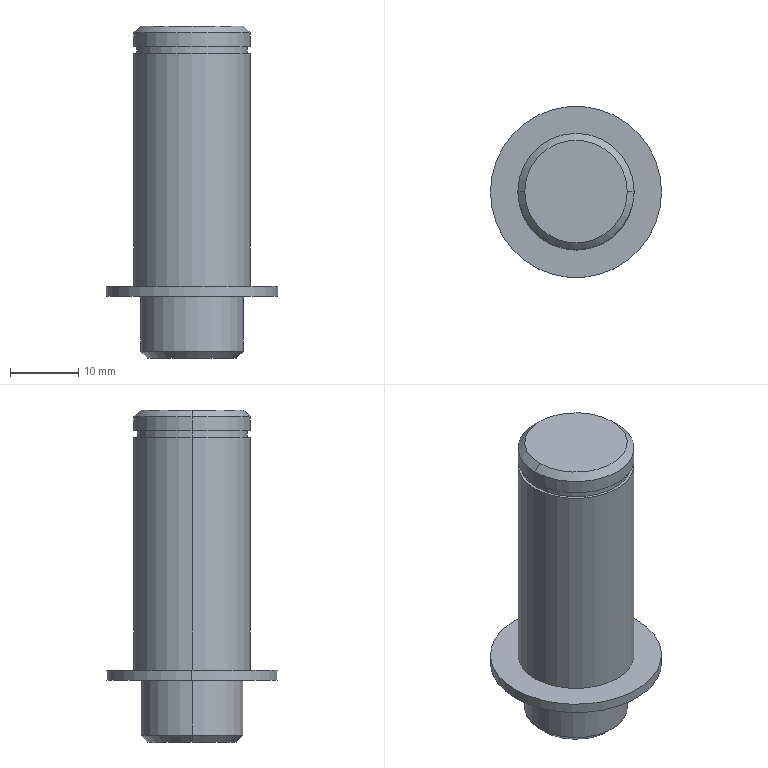Part | STEP file | CON-005 | 1 solid | 24 faces | box 25 x 25 x 48.5 mm | volume 10531 mm3 | cylinder 12 | cone 6 | plane 6 | commonest cylinder face diameters 17 x4 4.2 x2 15 x2 16.2 x2 25 x2
STEP:
#1=CARTESIAN_POINT('',(0.,0.,0.));
#2=DIRECTION('',(0.,0.,1.));
#3=DIRECTION('',(1.,0.,0.));
#4=AXIS2_PLACEMENT_3D('',#1,#2,#3);
#5=CARTESIAN_POINT('',(-6.5,0.,-44.5));
#6=VERTEX_POINT('',#5);
#7=CARTESIAN_POINT('',(6.5,0.,-44.5));
#8=VERTEX_POINT('',#7);
#9=CARTESIAN_POINT('',(0.,0.,-44.5));
#10=DIRECTION('',(0.,0.,-1.));
#11=DIRECTION('',(-1.,0.,0.));
#12=AXIS2_PLACEMENT_3D('',#9,#10,#11);
#13=CIRCLE('',#12,6.5);
#14=CARTESIAN_POINT('',(0.,0.,-44.5));
#15=DIRECTION('',(0.,0.,1.));
#16=DIRECTION('',(1.,0.,0.));
#17=AXIS2_PLACEMENT_3D('',#14,#15,#16);
#18=CONICAL_SURFACE('',#17,6.5,0.7854);
#19=CARTESIAN_POINT('',(3.142,0.));
#20=DIRECTION('',(-1.,0.));
#21=VECTOR('',#20,1.);
#22=LINE('',#19,#21);
#23=(GEOMETRIC_REPRESENTATION_CONTEXT(2)PARAMETRIC_REPRESENTATION_CONTEXT()REPRESENTATION_CONTEXT('',''));
#24=DEFINITIONAL_REPRESENTATION('',(#22),#23);
#25=PCURVE('',#18,#24);
#26=CARTESIAN_POINT('',(0.,0.,-44.5));
#27=DIRECTION('',(0.,0.,-1.));
#28=DIRECTION('',(-1.,0.,0.));
#29=AXIS2_PLACEMENT_3D('',#26,#27,#28);
#30=PLANE('',#29);
#31=CARTESIAN_POINT('',(0.,0.));
#32=DIRECTION('',(1.,0.));
#33=AXIS2_PLACEMENT_2D('',#31,#32);
#34=CIRCLE('',#33,6.5);
#35=(GEOMETRIC_REPRESENTATION_CONTEXT(2)PARAMETRIC_REPRESENTATION_CONTEXT()REPRESENTATION_CONTEXT('',''));
#36=DEFINITIONAL_REPRESENTATION('',(#34),#35);
#37=PCURVE('',#30,#36);
#38=SURFACE_CURVE('',#13,(#25,#37),.PCURVE_S1.);
#39=EDGE_CURVE('',#6,#8,#38,.T.);
#40=ORIENTED_EDGE('',*,*,#39,.F.);
#41=CARTESIAN_POINT('',(-7.5,0.,-43.5));
#42=VERTEX_POINT('',#41);
#43=CARTESIAN_POINT('',(-6.5,0.,-44.5));
#44=DIRECTION('',(-0.7071,0.,0.7071));
#45=VECTOR('',#44,1.);
#46=LINE('',#43,#45);
#47=CARTESIAN_POINT('',(3.142,0.));
#48=DIRECTION('',(0.,1.));
#49=VECTOR('',#48,1.);
#50=LINE('',#47,#49);
#51=(GEOMETRIC_REPRESENTATION_CONTEXT(2)PARAMETRIC_REPRESENTATION_CONTEXT()REPRESENTATION_CONTEXT('',''));
#52=DEFINITIONAL_REPRESENTATION('',(#50),#51);
#53=PCURVE('',#18,#52);
#54=CARTESIAN_POINT('',(0.,0.,-44.5));
#55=DIRECTION('',(0.,0.,1.));
#56=DIRECTION('',(1.,0.,0.));
#57=AXIS2_PLACEMENT_3D('',#54,#55,#56);
#58=CONICAL_SURFACE('',#57,6.5,0.7854);
#59=CARTESIAN_POINT('',(3.142,0.));
#60=DIRECTION('',(0.,1.));
#61=VECTOR('',#60,1.);
#62=LINE('',#59,#61);
#63=(GEOMETRIC_REPRESENTATION_CONTEXT(2)PARAMETRIC_REPRESENTATION_CONTEXT()REPRESENTATION_CONTEXT('',''));
#64=DEFINITIONAL_REPRESENTATION('',(#62),#63);
#65=PCURVE('',#58,#64);
#66=SURFACE_CURVE('',#46,(#53,#65),.PCURVE_S1.);
#67=EDGE_CURVE('',#6,#42,#66,.T.);
#68=ORIENTED_EDGE('',*,*,#67,.T.);
#69=CARTESIAN_POINT('',(7.5,0.,-43.5));
#70=VERTEX_POINT('',#69);
#71=CARTESIAN_POINT('',(0.,0.,-43.5));
#72=DIRECTION('',(0.,0.,1.));
#73=DIRECTION('',(-1.,0.,0.));
#74=AXIS2_PLACEMENT_3D('',#71,#72,#73);
#75=CIRCLE('',#74,7.5);
#76=CARTESIAN_POINT('',(-3.142,1.));
#77=DIRECTION('',(1.,0.));
#78=VECTOR('',#77,1.);
#79=LINE('',#76,#78);
#80=(GEOMETRIC_REPRESENTATION_CONTEXT(2)PARAMETRIC_REPRESENTATION_CONTEXT()REPRESENTATION_CONTEXT('',''));
#81=DEFINITIONAL_REPRESENTATION('',(#79),#80);
#82=PCURVE('',#18,#81);
#83=CARTESIAN_POINT('',(0.,0.,-44.5));
#84=DIRECTION('',(0.,0.,1.));
#85=DIRECTION('',(1.,0.,0.));
#86=AXIS2_PLACEMENT_3D('',#83,#84,#85);
#87=CYLINDRICAL_SURFACE('',#86,7.5);
#88=CARTESIAN_POINT('',(-3.142,1.));
#89=DIRECTION('',(1.,0.));
#90=VECTOR('',#89,1.);
#91=LINE('',#88,#90);
#92=(GEOMETRIC_REPRESENTATION_CONTEXT(2)PARAMETRIC_REPRESENTATION_CONTEXT()REPRESENTATION_CONTEXT('',''));
#93=DEFINITIONAL_REPRESENTATION('',(#91),#92);
#94=PCURVE('',#87,#93);
#95=SURFACE_CURVE('',#75,(#82,#94),.PCURVE_S1.);
#96=EDGE_CURVE('',#70,#42,#95,.T.);
#97=ORIENTED_EDGE('',*,*,#96,.F.);
#98=CARTESIAN_POINT('',(6.5,0.,-44.5));
#99=DIRECTION('',(0.7071,0.,0.7071));
#100=VECTOR('',#99,1.);
#101=LINE('',#98,#100);
#102=CARTESIAN_POINT('',(0.,0.));
#103=DIRECTION('',(0.,1.));
#104=VECTOR('',#103,1.);
#105=LINE('',#102,#104);
#106=(GEOMETRIC_REPRESENTATION_CONTEXT(2)PARAMETRIC_REPRESENTATION_CONTEXT()REPRESENTATION_CONTEXT('',''));
#107=DEFINITIONAL_REPRESENTATION('',(#105),#106);
#108=PCURVE('',#18,#107);
#109=CARTESIAN_POINT('',(6.283,0.));
#110=DIRECTION('',(0.,1.));
#111=VECTOR('',#110,1.);
#112=LINE('',#109,#111);
#113=(GEOMETRIC_REPRESENTATION_CONTEXT(2)PARAMETRIC_REPRESENTATION_CONTEXT()REPRESENTATION_CONTEXT('',''));
#114=DEFINITIONAL_REPRESENTATION('',(#112),#113);
#115=PCURVE('',#58,#114);
#116=SURFACE_CURVE('',#101,(#108,#115),.PCURVE_S1.);
#117=EDGE_CURVE('',#8,#70,#116,.T.);
#118=ORIENTED_EDGE('',*,*,#117,.F.);
#119=EDGE_LOOP('',(#40,#68,#97,#118));
#120=FACE_BOUND('',#119,.T.);
#121=ADVANCED_FACE('',(#120),#18,.T.);
#122=CARTESIAN_POINT('',(7.5,0.,4.));
#123=VERTEX_POINT('',#122);
#124=CARTESIAN_POINT('',(-7.5,0.,4.));
#125=VERTEX_POINT('',#124);
#126=CARTESIAN_POINT('',(0.,0.,4.));
#127=DIRECTION('',(0.,0.,1.));
#128=DIRECTION('',(1.,0.,0.));
#129=AXIS2_PLACEMENT_3D('',#126,#127,#128);
#130=CIRCLE('',#129,7.5);
#131=CARTESIAN_POINT('',(0.,0.,4.));
#132=DIRECTION('',(0.,0.,-1.));
#133=DIRECTION('',(-1.,0.,0.));
#134=AXIS2_PLACEMENT_3D('',#131,#132,#133);
#135=CONICAL_SURFACE('',#134,7.5,0.7854);
#136=CARTESIAN_POINT('',(3.142,0.));
#137=DIRECTION('',(-1.,0.));
#138=VECTOR('',#137,1.);
#139=LINE('',#136,#138);
#140=(GEOMETRIC_REPRESENTATION_CONTEXT(2)PARAMETRIC_REPRESENTATION_CONTEXT()REPRESENTATION_CONTEXT('',''));
#141=DEFINITIONAL_REPRESENTATION('',(#139),#140);
#142=PCURVE('',#135,#141);
#143=CARTESIAN_POINT('',(0.,0.,4.));
#144=DIRECTION('',(0.,0.,1.));
#145=DIRECTION('',(1.,0.,0.));
#146=AXIS2_PLACEMENT_3D('',#143,#144,#145);
#147=PLANE('',#146);
#148=CARTESIAN_POINT('',(0.,0.));
#149=DIRECTION('',(1.,0.));
#150=AXIS2_PLACEMENT_2D('',#148,#149);
#151=CIRCLE('',#150,7.5);
#152=(GEOMETRIC_REPRESENTATION_CONTEXT(2)PARAMETRIC_REPRESENTATION_CONTEXT()REPRESENTATION_CONTEXT('',''));
#153=DEFINITIONAL_REPRESENTATION('',(#151),#152);
#154=PCURVE('',#147,#153);
#155=SURFACE_CURVE('',#130,(#142,#154),.PCURVE_S1.);
#156=EDGE_CURVE('',#123,#125,#155,.T.);
#157=ORIENTED_EDGE('',*,*,#156,.F.);
#158=CARTESIAN_POINT('',(8.5,0.,3.));
#159=VERTEX_POINT('',#158);
#160=CARTESIAN_POINT('',(7.5,0.,4.));
#161=DIRECTION('',(0.7071,0.,-0.7071));
#162=VECTOR('',#161,1.);
#163=LINE('',#160,#162);
#164=CARTESIAN_POINT('',(3.142,0.));
#165=DIRECTION('',(0.,1.));
#166=VECTOR('',#165,1.);
#167=LINE('',#164,#166);
#168=(GEOMETRIC_REPRESENTATION_CONTEXT(2)PARAMETRIC_REPRESENTATION_CONTEXT()REPRESENTATION_CONTEXT('',''));
#169=DEFINITIONAL_REPRESENTATION('',(#167),#168);
#170=PCURVE('',#135,#169);
#171=CARTESIAN_POINT('',(0.,0.,4.));
#172=DIRECTION('',(0.,0.,-1.));
#173=DIRECTION('',(-1.,0.,0.));
#174=AXIS2_PLACEMENT_3D('',#171,#172,#173);
#175=CONICAL_SURFACE('',#174,7.5,0.7854);
#176=CARTESIAN_POINT('',(3.142,0.));
#177=DIRECTION('',(0.,1.));
#178=VECTOR('',#177,1.);
#179=LINE('',#176,#178);
#180=(GEOMETRIC_REPRESENTATION_CONTEXT(2)PARAMETRIC_REPRESENTATION_CONTEXT()REPRESENTATION_CONTEXT('',''));
#181=DEFINITIONAL_REPRESENTATION('',(#179),#180);
#182=PCURVE('',#175,#181);
#183=SURFACE_CURVE('',#163,(#170,#182),.PCURVE_S1.);
#184=EDGE_CURVE('',#123,#159,#183,.T.);
#185=ORIENTED_EDGE('',*,*,#184,.T.);
#186=CARTESIAN_POINT('',(-8.5,0.,3.));
#187=VERTEX_POINT('',#186);
#188=CARTESIAN_POINT('',(0.,0.,3.));
#189=DIRECTION('',(0.,0.,-1.));
#190=DIRECTION('',(1.,0.,0.));
#191=AXIS2_PLACEMENT_3D('',#188,#189,#190);
#192=CIRCLE('',#191,8.5);
#193=CARTESIAN_POINT('',(-3.142,1.));
#194=DIRECTION('',(1.,0.));
#195=VECTOR('',#194,1.);
#196=LINE('',#193,#195);
#197=(GEOMETRIC_REPRESENTATION_CONTEXT(2)PARAMETRIC_REPRESENTATION_CONTEXT()REPRESENTATION_CONTEXT('',''));
#198=DEFINITIONAL_REPRESENTATION('',(#196),#197);
#199=PCURVE('',#135,#198);
#200=CARTESIAN_POINT('',(0.,0.,4.));
#201=DIRECTION('',(0.,0.,-1.));
#202=DIRECTION('',(-1.,0.,0.));
#203=AXIS2_PLACEMENT_3D('',#200,#201,#202);
#204=CYLINDRICAL_SURFACE('',#203,8.5);
#205=CARTESIAN_POINT('',(-3.142,1.));
#206=DIRECTION('',(1.,0.));
#207=VECTOR('',#206,1.);
#208=LINE('',#205,#207);
#209=(GEOMETRIC_REPRESENTATION_CONTEXT(2)PARAMETRIC_REPRESENTATION_CONTEXT()REPRESENTATION_CONTEXT('',''));
#210=DEFINITIONAL_REPRESENTATION('',(#208),#209);
#211=PCURVE('',#204,#210);
#212=SURFACE_CURVE('',#192,(#199,#211),.PCURVE_S1.);
#213=EDGE_CURVE('',#187,#159,#212,.T.);
#214=ORIENTED_EDGE('',*,*,#213,.F.);
#215=CARTESIAN_POINT('',(-7.5,0.,4.));
#216=DIRECTION('',(-0.7071,0.,-0.7071));
#217=VECTOR('',#216,1.);
#218=LINE('',#215,#217);
#219=CARTESIAN_POINT('',(0.,0.));
#220=DIRECTION('',(0.,1.));
#221=VECTOR('',#220,1.);
#222=LINE('',#219,#221);
#223=(GEOMETRIC_REPRESENTATION_CONTEXT(2)PARAMETRIC_REPRESENTATION_CONTEXT()REPRESENTATION_CONTEXT('',''));
#224=DEFINITIONAL_REPRESENTATION('',(#222),#223);
#225=PCURVE('',#135,#224);
#226=CARTESIAN_POINT('',(6.283,0.));
#227=DIRECTION('',(0.,1.));
#228=VECTOR('',#227,1.);
#229=LINE('',#226,#228);
#230=(GEOMETRIC_REPRESENTATION_CONTEXT(2)PARAMETRIC_REPRESENTATION_CONTEXT()REPRESENTATION_CONTEXT('',''));
#231=DEFINITIONAL_REPRESENTATION('',(#229),#230);
#232=PCURVE('',#175,#231);
#233=SURFACE_CURVE('',#218,(#225,#232),.PCURVE_S1.);
#234=EDGE_CURVE('',#125,#187,#233,.T.);
#235=ORIENTED_EDGE('',*,*,#234,.F.);
#236=EDGE_LOOP('',(#157,#185,#214,#235));
#237=FACE_BOUND('',#236,.T.);
#238=ADVANCED_FACE('',(#237),#135,.T.);
#239=CARTESIAN_POINT('',(-2.1,0.,-19.5));
#240=VERTEX_POINT('',#239);
#241=CARTESIAN_POINT('',(-2.1,0.,-44.5));
#242=VERTEX_POINT('',#241);
#243=CARTESIAN_POINT('',(-2.1,0.,-44.5));
#244=DIRECTION('',(0.,0.,-1.));
#245=VECTOR('',#244,1.);
#246=LINE('',#243,#245);
#247=CARTESIAN_POINT('',(0.,0.,-44.5));
#248=DIRECTION('',(0.,0.,-1.));
#249=DIRECTION('',(-1.,0.,0.));
#250=AXIS2_PLACEMENT_3D('',#247,#248,#249);
#251=CYLINDRICAL_SURFACE('',#250,2.1);
#252=CARTESIAN_POINT('',(6.283,0.));
#253=DIRECTION('',(0.,1.));
#254=VECTOR('',#253,1.);
#255=LINE('',#252,#254);
#256=(GEOMETRIC_REPRESENTATION_CONTEXT(2)PARAMETRIC_REPRESENTATION_CONTEXT()REPRESENTATION_CONTEXT('',''));
#257=DEFINITIONAL_REPRESENTATION('',(#255),#256);
#258=PCURVE('',#251,#257);
#259=CARTESIAN_POINT('',(0.,0.,-44.5));
#260=DIRECTION('',(0.,0.,-1.));
#261=DIRECTION('',(-1.,0.,0.));
#262=AXIS2_PLACEMENT_3D('',#259,#260,#261);
#263=CYLINDRICAL_SURFACE('',#262,2.1);
#264=CARTESIAN_POINT('',(0.,0.));
#265=DIRECTION('',(0.,1.));
#266=VECTOR('',#265,1.);
#267=LINE('',#264,#266);
#268=(GEOMETRIC_REPRESENTATION_CONTEXT(2)PARAMETRIC_REPRESENTATION_CONTEXT()REPRESENTATION_CONTEXT('',''));
#269=DEFINITIONAL_REPRESENTATION('',(#267),#268);
#270=PCURVE('',#263,#269);
#271=SURFACE_CURVE('',#246,(#258,#270),.PCURVE_S1.);
#272=EDGE_CURVE('',#240,#242,#271,.T.);
#273=ORIENTED_EDGE('',*,*,#272,.T.);
#274=CARTESIAN_POINT('',(2.1,0.,-44.5));
#275=VERTEX_POINT('',#274);
#276=CARTESIAN_POINT('',(0.,0.,-44.5));
#277=DIRECTION('',(0.,0.,-1.));
#278=DIRECTION('',(-1.,0.,0.));
#279=AXIS2_PLACEMENT_3D('',#276,#277,#278);
#280=CIRCLE('',#279,2.1);
#281=CARTESIAN_POINT('',(0.,0.));
#282=DIRECTION('',(1.,0.));
#283=VECTOR('',#282,1.);
#284=LINE('',#281,#283);
#285=(GEOMETRIC_REPRESENTATION_CONTEXT(2)PARAMETRIC_REPRESENTATION_CONTEXT()REPRESENTATION_CONTEXT('',''));
#286=DEFINITIONAL_REPRESENTATION('',(#284),#285);
#287=PCURVE('',#251,#286);
#288=CARTESIAN_POINT('',(0.,0.));
#289=DIRECTION('',(1.,0.));
#290=AXIS2_PLACEMENT_2D('',#288,#289);
#291=CIRCLE('',#290,2.1);
#292=(GEOMETRIC_REPRESENTATION_CONTEXT(2)PARAMETRIC_REPRESENTATION_CONTEXT()REPRESENTATION_CONTEXT('',''));
#293=DEFINITIONAL_REPRESENTATION('',(#291),#292);
#294=PCURVE('',#30,#293);
#295=SURFACE_CURVE('',#280,(#287,#294),.PCURVE_S1.);
#296=EDGE_CURVE('',#275,#242,#295,.T.);
#297=ORIENTED_EDGE('',*,*,#296,.F.);
#298=CARTESIAN_POINT('',(2.1,0.,-19.5));
#299=VERTEX_POINT('',#298);
#300=CARTESIAN_POINT('',(2.1,0.,-44.5));
#301=DIRECTION('',(0.,0.,-1.));
#302=VECTOR('',#301,1.);
#303=LINE('',#300,#302);
#304=CARTESIAN_POINT('',(3.142,0.));
#305=DIRECTION('',(0.,1.));
#306=VECTOR('',#305,1.);
#307=LINE('',#304,#306);
#308=(GEOMETRIC_REPRESENTATION_CONTEXT(2)PARAMETRIC_REPRESENTATION_CONTEXT()REPRESENTATION_CONTEXT('',''));
#309=DEFINITIONAL_REPRESENTATION('',(#307),#308);
#310=PCURVE('',#251,#309);
#311=CARTESIAN_POINT('',(3.142,0.));
#312=DIRECTION('',(0.,1.));
#313=VECTOR('',#312,1.);
#314=LINE('',#311,#313);
#315=(GEOMETRIC_REPRESENTATION_CONTEXT(2)PARAMETRIC_REPRESENTATION_CONTEXT()REPRESENTATION_CONTEXT('',''));
#316=DEFINITIONAL_REPRESENTATION('',(#314),#315);
#317=PCURVE('',#263,#316);
#318=SURFACE_CURVE('',#303,(#310,#317),.PCURVE_S1.);
#319=EDGE_CURVE('',#299,#275,#318,.T.);
#320=ORIENTED_EDGE('',*,*,#319,.F.);
#321=CARTESIAN_POINT('',(0.,0.,-19.5));
#322=DIRECTION('',(0.,0.,-1.));
#323=DIRECTION('',(-1.,0.,0.));
#324=AXIS2_PLACEMENT_3D('',#321,#322,#323);
#325=CIRCLE('',#324,2.1);
#326=CARTESIAN_POINT('',(0.,-25.));
#327=DIRECTION('',(1.,0.));
#328=VECTOR('',#327,1.);
#329=LINE('',#326,#328);
#330=(GEOMETRIC_REPRESENTATION_CONTEXT(2)PARAMETRIC_REPRESENTATION_CONTEXT()REPRESENTATION_CONTEXT('',''));
#331=DEFINITIONAL_REPRESENTATION('',(#329),#330);
#332=PCURVE('',#251,#331);
#333=CARTESIAN_POINT('',(0.,0.,-19.5));
#334=DIRECTION('',(0.,0.,-1.));
#335=DIRECTION('',(-1.,0.,0.));
#336=AXIS2_PLACEMENT_3D('',#333,#334,#335);
#337=CONICAL_SURFACE('',#336,2.1,1.03);
#338=CARTESIAN_POINT('',(0.,0.));
#339=DIRECTION('',(1.,0.));
#340=VECTOR('',#339,1.);
#341=LINE('',#338,#340);
#342=(GEOMETRIC_REPRESENTATION_CONTEXT(2)PARAMETRIC_REPRESENTATION_CONTEXT()REPRESENTATION_CONTEXT('',''));
#343=DEFINITIONAL_REPRESENTATION('',(#341),#342);
#344=PCURVE('',#337,#343);
#345=SURFACE_CURVE('',#325,(#332,#344),.PCURVE_S1.);
#346=EDGE_CURVE('',#299,#240,#345,.T.);
#347=ORIENTED_EDGE('',*,*,#346,.T.);
#348=EDGE_LOOP('',(#273,#297,#320,#347));
#349=FACE_BOUND('',#348,.F.);
#350=ADVANCED_FACE('',(#349),#251,.F.);
#351=ORIENTED_EDGE('',*,*,#346,.F.);
#352=CARTESIAN_POINT('',(0.,0.,-18.238));
#353=VERTEX_POINT('',#352);
#354=CARTESIAN_POINT('',(2.1,0.,-19.5));
#355=DIRECTION('',(0.8572,0.,-0.515));
#356=VECTOR('',#355,1.);
#357=LINE('',#354,#356);
#358=CARTESIAN_POINT('',(3.142,0.));
#359=DIRECTION('',(0.,1.));
#360=VECTOR('',#359,1.);
#361=LINE('',#358,#360);
#362=(GEOMETRIC_REPRESENTATION_CONTEXT(2)PARAMETRIC_REPRESENTATION_CONTEXT()REPRESENTATION_CONTEXT('',''));
#363=DEFINITIONAL_REPRESENTATION('',(#361),#362);
#364=PCURVE('',#337,#363);
#365=CARTESIAN_POINT('',(0.,0.,-19.5));
#366=DIRECTION('',(0.,0.,-1.));
#367=DIRECTION('',(-1.,0.,0.));
#368=AXIS2_PLACEMENT_3D('',#365,#366,#367);
#369=CONICAL_SURFACE('',#368,2.1,1.03);
#370=CARTESIAN_POINT('',(3.142,0.));
#371=DIRECTION('',(0.,1.));
#372=VECTOR('',#371,1.);
#373=LINE('',#370,#372);
#374=(GEOMETRIC_REPRESENTATION_CONTEXT(2)PARAMETRIC_REPRESENTATION_CONTEXT()REPRESENTATION_CONTEXT('',''));
#375=DEFINITIONAL_REPRESENTATION('',(#373),#374);
#376=PCURVE('',#369,#375);
#377=SURFACE_CURVE('',#357,(#364,#376),.PCURVE_S1.);
#378=EDGE_CURVE('',#353,#299,#377,.T.);
#379=ORIENTED_EDGE('',*,*,#378,.F.);
#380=CARTESIAN_POINT('',(-2.1,0.,-19.5));
#381=DIRECTION('',(-0.8572,0.,-0.515));
#382=VECTOR('',#381,1.);
#383=LINE('',#380,#382);
#384=CARTESIAN_POINT('',(6.283,0.));
#385=DIRECTION('',(0.,1.));
#386=VECTOR('',#385,1.);
#387=LINE('',#384,#386);
#388=(GEOMETRIC_REPRESENTATION_CONTEXT(2)PARAMETRIC_REPRESENTATION_CONTEXT()REPRESENTATION_CONTEXT('',''));
#389=DEFINITIONAL_REPRESENTATION('',(#387),#388);
#390=PCURVE('',#337,#389);
#391=CARTESIAN_POINT('',(0.,0.));
#392=DIRECTION('',(0.,1.));
#393=VECTOR('',#392,1.);
#394=LINE('',#391,#393);
#395=(GEOMETRIC_REPRESENTATION_CONTEXT(2)PARAMETRIC_REPRESENTATION_CONTEXT()REPRESENTATION_CONTEXT('',''));
#396=DEFINITIONAL_REPRESENTATION('',(#394),#395);
#397=PCURVE('',#369,#396);
#398=SURFACE_CURVE('',#383,(#390,#397),.PCURVE_S1.);
#399=EDGE_CURVE('',#353,#240,#398,.T.);
#400=ORIENTED_EDGE('',*,*,#399,.T.);
#401=EDGE_LOOP('',(#351,#379,#400));
#402=FACE_BOUND('',#401,.F.);
#403=ADVANCED_FACE('',(#402),#337,.F.);
#404=ORIENTED_EDGE('',*,*,#213,.T.);
#405=CARTESIAN_POINT('',(8.5,0.,1.));
#406=VERTEX_POINT('',#405);
#407=CARTESIAN_POINT('',(8.5,0.,4.));
#408=DIRECTION('',(0.,0.,-1.));
#409=VECTOR('',#408,1.);
#410=LINE('',#407,#409);
#411=CARTESIAN_POINT('',(3.142,0.));
#412=DIRECTION('',(0.,1.));
#413=VECTOR('',#412,1.);
#414=LINE('',#411,#413);
#415=(GEOMETRIC_REPRESENTATION_CONTEXT(2)PARAMETRIC_REPRESENTATION_CONTEXT()REPRESENTATION_CONTEXT('',''));
#416=DEFINITIONAL_REPRESENTATION('',(#414),#415);
#417=PCURVE('',#204,#416);
#418=CARTESIAN_POINT('',(0.,0.,4.));
#419=DIRECTION('',(0.,0.,-1.));
#420=DIRECTION('',(-1.,0.,0.));
#421=AXIS2_PLACEMENT_3D('',#418,#419,#420);
#422=CYLINDRICAL_SURFACE('',#421,8.5);
#423=CARTESIAN_POINT('',(3.142,0.));
#424=DIRECTION('',(0.,1.));
#425=VECTOR('',#424,1.);
#426=LINE('',#423,#425);
#427=(GEOMETRIC_REPRESENTATION_CONTEXT(2)PARAMETRIC_REPRESENTATION_CONTEXT()REPRESENTATION_CONTEXT('',''));
#428=DEFINITIONAL_REPRESENTATION('',(#426),#427);
#429=PCURVE('',#422,#428);
#430=SURFACE_CURVE('',#410,(#417,#429),.PCURVE_S1.);
#431=EDGE_CURVE('',#159,#406,#430,.T.);
#432=ORIENTED_EDGE('',*,*,#431,.T.);
#433=CARTESIAN_POINT('',(-8.5,0.,1.));
#434=VERTEX_POINT('',#433);
#435=CARTESIAN_POINT('',(0.,0.,1.));
#436=DIRECTION('',(0.,0.,1.));
#437=DIRECTION('',(1.,0.,0.));
#438=AXIS2_PLACEMENT_3D('',#435,#436,#437);
#439=CIRCLE('',#438,8.5);
#440=CARTESIAN_POINT('',(3.142,3.));
#441=DIRECTION('',(-1.,0.));
#442=VECTOR('',#441,1.);
#443=LINE('',#440,#442);
#444=(GEOMETRIC_REPRESENTATION_CONTEXT(2)PARAMETRIC_REPRESENTATION_CONTEXT()REPRESENTATION_CONTEXT('',''));
#445=DEFINITIONAL_REPRESENTATION('',(#443),#444);
#446=PCURVE('',#204,#445);
#447=CARTESIAN_POINT('',(0.,0.,1.));
#448=DIRECTION('',(0.,0.,1.));
#449=DIRECTION('',(1.,0.,0.));
#450=AXIS2_PLACEMENT_3D('',#447,#448,#449);
#451=PLANE('',#450);
#452=CARTESIAN_POINT('',(0.,0.));
#453=DIRECTION('',(1.,0.));
#454=AXIS2_PLACEMENT_2D('',#452,#453);
#455=CIRCLE('',#454,8.5);
#456=(GEOMETRIC_REPRESENTATION_CONTEXT(2)PARAMETRIC_REPRESENTATION_CONTEXT()REPRESENTATION_CONTEXT('',''));
#457=DEFINITIONAL_REPRESENTATION('',(#455),#456);
#458=PCURVE('',#451,#457);
#459=SURFACE_CURVE('',#439,(#446,#458),.PCURVE_S1.);
#460=EDGE_CURVE('',#406,#434,#459,.T.);
#461=ORIENTED_EDGE('',*,*,#460,.T.);
#462=CARTESIAN_POINT('',(-8.5,0.,4.));
#463=DIRECTION('',(0.,0.,-1.));
#464=VECTOR('',#463,1.);
#465=LINE('',#462,#464);
#466=CARTESIAN_POINT('',(0.,0.));
#467=DIRECTION('',(0.,1.));
#468=VECTOR('',#467,1.);
#469=LINE('',#466,#468);
#470=(GEOMETRIC_REPRESENTATION_CONTEXT(2)PARAMETRIC_REPRESENTATION_CONTEXT()REPRESENTATION_CONTEXT('',''));
#471=DEFINITIONAL_REPRESENTATION('',(#469),#470);
#472=PCURVE('',#204,#471);
#473=CARTESIAN_POINT('',(6.283,0.));
#474=DIRECTION('',(0.,1.));
#475=VECTOR('',#474,1.);
#476=LINE('',#473,#475);
#477=(GEOMETRIC_REPRESENTATION_CONTEXT(2)PARAMETRIC_REPRESENTATION_CONTEXT()REPRESENTATION_CONTEXT('',''));
#478=DEFINITIONAL_REPRESENTATION('',(#476),#477);
#479=PCURVE('',#422,#478);
#480=SURFACE_CURVE('',#465,(#472,#479),.PCURVE_S1.);
#481=EDGE_CURVE('',#187,#434,#480,.T.);
#482=ORIENTED_EDGE('',*,*,#481,.F.);
#483=EDGE_LOOP('',(#404,#432,#461,#482));
#484=FACE_BOUND('',#483,.T.);
#485=ADVANCED_FACE('',(#484),#204,.T.);
#486=CARTESIAN_POINT('',(8.1,0.,1.));
#487=VERTEX_POINT('',#486);
#488=CARTESIAN_POINT('',(-8.1,0.,1.));
#489=VERTEX_POINT('',#488);
#490=CARTESIAN_POINT('',(0.,0.,1.));
#491=DIRECTION('',(0.,0.,1.));
#492=DIRECTION('',(1.,0.,0.));
#493=AXIS2_PLACEMENT_3D('',#490,#491,#492);
#494=CIRCLE('',#493,8.1);
#495=CARTESIAN_POINT('',(0.,0.,1.));
#496=DIRECTION('',(0.,0.,-1.));
#497=DIRECTION('',(-1.,0.,0.));
#498=AXIS2_PLACEMENT_3D('',#495,#496,#497);
#499=CYLINDRICAL_SURFACE('',#498,8.1);
#500=CARTESIAN_POINT('',(3.142,0.));
#501=DIRECTION('',(-1.,0.));
#502=VECTOR('',#501,1.);
#503=LINE('',#500,#502);
#504=(GEOMETRIC_REPRESENTATION_CONTEXT(2)PARAMETRIC_REPRESENTATION_CONTEXT()REPRESENTATION_CONTEXT('',''));
#505=DEFINITIONAL_REPRESENTATION('',(#503),#504);
#506=PCURVE('',#499,#505);
#507=CARTESIAN_POINT('',(0.,0.));
#508=DIRECTION('',(1.,0.));
#509=AXIS2_PLACEMENT_2D('',#507,#508);
#510=CIRCLE('',#509,8.1);
#511=(GEOMETRIC_REPRESENTATION_CONTEXT(2)PARAMETRIC_REPRESENTATION_CONTEXT()REPRESENTATION_CONTEXT('',''));
#512=DEFINITIONAL_REPRESENTATION('',(#510),#511);
#513=PCURVE('',#451,#512);
#514=SURFACE_CURVE('',#494,(#506,#513),.PCURVE_S1.);
#515=EDGE_CURVE('',#487,#489,#514,.T.);
#516=ORIENTED_EDGE('',*,*,#515,.F.);
#517=CARTESIAN_POINT('',(8.1,0.,0.));
#518=VERTEX_POINT('',#517);
#519=CARTESIAN_POINT('',(8.1,0.,1.));
#520=DIRECTION('',(0.,0.,-1.));
#521=VECTOR('',#520,1.);
#522=LINE('',#519,#521);
#523=CARTESIAN_POINT('',(3.142,0.));
#524=DIRECTION('',(0.,1.));
#525=VECTOR('',#524,1.);
#526=LINE('',#523,#525);
#527=(GEOMETRIC_REPRESENTATION_CONTEXT(2)PARAMETRIC_REPRESENTATION_CONTEXT()REPRESENTATION_CONTEXT('',''));
#528=DEFINITIONAL_REPRESENTATION('',(#526),#527);
#529=PCURVE('',#499,#528);
#530=CARTESIAN_POINT('',(0.,0.,1.));
#531=DIRECTION('',(0.,0.,-1.));
#532=DIRECTION('',(-1.,0.,0.));
#533=AXIS2_PLACEMENT_3D('',#530,#531,#532);
#534=CYLINDRICAL_SURFACE('',#533,8.1);
#535=CARTESIAN_POINT('',(3.142,0.));
#536=DIRECTION('',(0.,1.));
#537=VECTOR('',#536,1.);
#538=LINE('',#535,#537);
#539=(GEOMETRIC_REPRESENTATION_CONTEXT(2)PARAMETRIC_REPRESENTATION_CONTEXT()REPRESENTATION_CONTEXT('',''));
#540=DEFINITIONAL_REPRESENTATION('',(#538),#539);
#541=PCURVE('',#534,#540);
#542=SURFACE_CURVE('',#522,(#529,#541),.PCURVE_S1.);
#543=EDGE_CURVE('',#487,#518,#542,.T.);
#544=ORIENTED_EDGE('',*,*,#543,.T.);
#545=CARTESIAN_POINT('',(-8.1,0.,0.));
#546=VERTEX_POINT('',#545);
#547=CARTESIAN_POINT('',(0.,0.,0.));
#548=DIRECTION('',(0.,0.,1.));
#549=DIRECTION('',(1.,0.,0.));
#550=AXIS2_PLACEMENT_3D('',#547,#548,#549);
#551=CIRCLE('',#550,8.1);
#552=CARTESIAN_POINT('',(3.142,1.));
#553=DIRECTION('',(-1.,0.));
#554=VECTOR('',#553,1.);
#555=LINE('',#552,#554);
#556=(GEOMETRIC_REPRESENTATION_CONTEXT(2)PARAMETRIC_REPRESENTATION_CONTEXT()REPRESENTATION_CONTEXT('',''));
#557=DEFINITIONAL_REPRESENTATION('',(#555),#556);
#558=PCURVE('',#499,#557);
#559=CARTESIAN_POINT('',(0.,0.,0.));
#560=DIRECTION('',(0.,0.,1.));
#561=DIRECTION('',(1.,0.,0.));
#562=AXIS2_PLACEMENT_3D('',#559,#560,#561);
#563=PLANE('',#562);
#564=CARTESIAN_POINT('',(0.,0.));
#565=DIRECTION('',(1.,0.));
#566=AXIS2_PLACEMENT_2D('',#564,#565);
#567=CIRCLE('',#566,8.1);
#568=(GEOMETRIC_REPRESENTATION_CONTEXT(2)PARAMETRIC_REPRESENTATION_CONTEXT()REPRESENTATION_CONTEXT('',''));
#569=DEFINITIONAL_REPRESENTATION('',(#567),#568);
#570=PCURVE('',#563,#569);
#571=SURFACE_CURVE('',#551,(#558,#570),.PCURVE_S1.);
#572=EDGE_CURVE('',#518,#546,#571,.T.);
#573=ORIENTED_EDGE('',*,*,#572,.T.);
#574=CARTESIAN_POINT('',(-8.1,0.,1.));
#575=DIRECTION('',(0.,0.,-1.));
#576=VECTOR('',#575,1.);
#577=LINE('',#574,#576);
#578=CARTESIAN_POINT('',(0.,0.));
#579=DIRECTION('',(0.,1.));
#580=VECTOR('',#579,1.);
#581=LINE('',#578,#580);
#582=(GEOMETRIC_REPRESENTATION_CONTEXT(2)PARAMETRIC_REPRESENTATION_CONTEXT()REPRESENTATION_CONTEXT('',''));
#583=DEFINITIONAL_REPRESENTATION('',(#581),#582);
#584=PCURVE('',#499,#583);
#585=CARTESIAN_POINT('',(6.283,0.));
#586=DIRECTION('',(0.,1.));
#587=VECTOR('',#586,1.);
#588=LINE('',#585,#587);
#589=(GEOMETRIC_REPRESENTATION_CONTEXT(2)PARAMETRIC_REPRESENTATION_CONTEXT()REPRESENTATION_CONTEXT('',''));
#590=DEFINITIONAL_REPRESENTATION('',(#588),#589);
#591=PCURVE('',#534,#590);
#592=SURFACE_CURVE('',#577,(#584,#591),.PCURVE_S1.);
#593=EDGE_CURVE('',#489,#546,#592,.T.);
#594=ORIENTED_EDGE('',*,*,#593,.F.);
#595=EDGE_LOOP('',(#516,#544,#573,#594));
#596=FACE_BOUND('',#595,.T.);
#597=ADVANCED_FACE('',(#596),#499,.T.);
#598=ORIENTED_EDGE('',*,*,#96,.T.);
#599=CARTESIAN_POINT('',(-7.5,0.,-35.5));
#600=VERTEX_POINT('',#599);
#601=CARTESIAN_POINT('',(-7.5,0.,-44.5));
#602=DIRECTION('',(0.,0.,1.));
#603=VECTOR('',#602,1.);
#604=LINE('',#601,#603);
#605=CARTESIAN_POINT('',(3.142,0.));
#606=DIRECTION('',(0.,1.));
#607=VECTOR('',#606,1.);
#608=LINE('',#605,#607);
#609=(GEOMETRIC_REPRESENTATION_CONTEXT(2)PARAMETRIC_REPRESENTATION_CONTEXT()REPRESENTATION_CONTEXT('',''));
#610=DEFINITIONAL_REPRESENTATION('',(#608),#609);
#611=PCURVE('',#87,#610);
#612=CARTESIAN_POINT('',(0.,0.,-44.5));
#613=DIRECTION('',(0.,0.,1.));
#614=DIRECTION('',(1.,0.,0.));
#615=AXIS2_PLACEMENT_3D('',#612,#613,#614);
#616=CYLINDRICAL_SURFACE('',#615,7.5);
#617=CARTESIAN_POINT('',(3.142,0.));
#618=DIRECTION('',(0.,1.));
#619=VECTOR('',#618,1.);
#620=LINE('',#617,#619);
#621=(GEOMETRIC_REPRESENTATION_CONTEXT(2)PARAMETRIC_REPRESENTATION_CONTEXT()REPRESENTATION_CONTEXT('',''));
#622=DEFINITIONAL_REPRESENTATION('',(#620),#621);
#623=PCURVE('',#616,#622);
#624=SURFACE_CURVE('',#604,(#611,#623),.PCURVE_S1.);
#625=EDGE_CURVE('',#42,#600,#624,.T.);
#626=ORIENTED_EDGE('',*,*,#625,.T.);
#627=CARTESIAN_POINT('',(7.5,0.,-35.5));
#628=VERTEX_POINT('',#627);
#629=CARTESIAN_POINT('',(0.,0.,-35.5));
#630=DIRECTION('',(0.,0.,-1.));
#631=DIRECTION('',(-1.,0.,0.));
#632=AXIS2_PLACEMENT_3D('',#629,#630,#631);
#633=CIRCLE('',#632,7.5);
#634=CARTESIAN_POINT('',(3.142,9.));
#635=DIRECTION('',(-1.,0.));
#636=VECTOR('',#635,1.);
#637=LINE('',#634,#636);
#638=(GEOMETRIC_REPRESENTATION_CONTEXT(2)PARAMETRIC_REPRESENTATION_CONTEXT()REPRESENTATION_CONTEXT('',''));
#639=DEFINITIONAL_REPRESENTATION('',(#637),#638);
#640=PCURVE('',#87,#639);
#641=CARTESIAN_POINT('',(0.,0.,-35.5));
#642=DIRECTION('',(0.,0.,-1.));
#643=DIRECTION('',(-1.,0.,0.));
#644=AXIS2_PLACEMENT_3D('',#641,#642,#643);
#645=PLANE('',#644);
#646=CARTESIAN_POINT('',(0.,0.));
#647=DIRECTION('',(1.,0.));
#648=AXIS2_PLACEMENT_2D('',#646,#647);
#649=CIRCLE('',#648,7.5);
#650=(GEOMETRIC_REPRESENTATION_CONTEXT(2)PARAMETRIC_REPRESENTATION_CONTEXT()REPRESENTATION_CONTEXT('',''));
#651=DEFINITIONAL_REPRESENTATION('',(#649),#650);
#652=PCURVE('',#645,#651);
#653=SURFACE_CURVE('',#633,(#640,#652),.PCURVE_S1.);
#654=EDGE_CURVE('',#600,#628,#653,.T.);
#655=ORIENTED_EDGE('',*,*,#654,.T.);
#656=CARTESIAN_POINT('',(7.5,0.,-44.5));
#657=DIRECTION('',(0.,0.,1.));
#658=VECTOR('',#657,1.);
#659=LINE('',#656,#658);
#660=CARTESIAN_POINT('',(0.,0.));
#661=DIRECTION('',(0.,1.));
#662=VECTOR('',#661,1.);
#663=LINE('',#660,#662);
#664=(GEOMETRIC_REPRESENTATION_CONTEXT(2)PARAMETRIC_REPRESENTATION_CONTEXT()REPRESENTATION_CONTEXT('',''));
#665=DEFINITIONAL_REPRESENTATION('',(#663),#664);
#666=PCURVE('',#87,#665);
#667=CARTESIAN_POINT('',(6.283,0.));
#668=DIRECTION('',(0.,1.));
#669=VECTOR('',#668,1.);
#670=LINE('',#667,#669);
#671=(GEOMETRIC_REPRESENTATION_CONTEXT(2)PARAMETRIC_REPRESENTATION_CONTEXT()REPRESENTATION_CONTEXT('',''));
#672=DEFINITIONAL_REPRESENTATION('',(#670),#671);
#673=PCURVE('',#616,#672);
#674=SURFACE_CURVE('',#659,(#666,#673),.PCURVE_S1.);
#675=EDGE_CURVE('',#70,#628,#674,.T.);
#676=ORIENTED_EDGE('',*,*,#675,.F.);
#677=EDGE_LOOP('',(#598,#626,#655,#676));
#678=FACE_BOUND('',#677,.T.);
#679=ADVANCED_FACE('',(#678),#87,.T.);
#680=CARTESIAN_POINT('',(-12.5,0.,-35.5));
#681=VERTEX_POINT('',#680);
#682=CARTESIAN_POINT('',(12.5,0.,-35.5));
#683=VERTEX_POINT('',#682);
#684=CARTESIAN_POINT('',(0.,0.,-35.5));
#685=DIRECTION('',(0.,0.,-1.));
#686=DIRECTION('',(-1.,0.,0.));
#687=AXIS2_PLACEMENT_3D('',#684,#685,#686);
#688=CIRCLE('',#687,12.5);
#689=CARTESIAN_POINT('',(0.,0.,-35.5));
#690=DIRECTION('',(0.,0.,1.));
#691=DIRECTION('',(1.,0.,0.));
#692=AXIS2_PLACEMENT_3D('',#689,#690,#691);
#693=CYLINDRICAL_SURFACE('',#692,12.5);
#694=CARTESIAN_POINT('',(3.142,0.));
#695=DIRECTION('',(-1.,0.));
#696=VECTOR('',#695,1.);
#697=LINE('',#694,#696);
#698=(GEOMETRIC_REPRESENTATION_CONTEXT(2)PARAMETRIC_REPRESENTATION_CONTEXT()REPRESENTATION_CONTEXT('',''));
#699=DEFINITIONAL_REPRESENTATION('',(#697),#698);
#700=PCURVE('',#693,#699);
#701=CARTESIAN_POINT('',(0.,0.));
#702=DIRECTION('',(1.,0.));
#703=AXIS2_PLACEMENT_2D('',#701,#702);
#704=CIRCLE('',#703,12.5);
#705=(GEOMETRIC_REPRESENTATION_CONTEXT(2)PARAMETRIC_REPRESENTATION_CONTEXT()REPRESENTATION_CONTEXT('',''));
#706=DEFINITIONAL_REPRESENTATION('',(#704),#705);
#707=PCURVE('',#645,#706);
#708=SURFACE_CURVE('',#688,(#700,#707),.PCURVE_S1.);
#709=EDGE_CURVE('',#681,#683,#708,.T.);
#710=ORIENTED_EDGE('',*,*,#709,.F.);
#711=CARTESIAN_POINT('',(-12.5,0.,-34.));
#712=VERTEX_POINT('',#711);
#713=CARTESIAN_POINT('',(-12.5,0.,-35.5));
#714=DIRECTION('',(0.,0.,1.));
#715=VECTOR('',#714,1.);
#716=LINE('',#713,#715);
#717=CARTESIAN_POINT('',(3.142,0.));
#718=DIRECTION('',(0.,1.));
#719=VECTOR('',#718,1.);
#720=LINE('',#717,#719);
#721=(GEOMETRIC_REPRESENTATION_CONTEXT(2)PARAMETRIC_REPRESENTATION_CONTEXT()REPRESENTATION_CONTEXT('',''));
#722=DEFINITIONAL_REPRESENTATION('',(#720),#721);
#723=PCURVE('',#693,#722);
#724=CARTESIAN_POINT('',(0.,0.,-35.5));
#725=DIRECTION('',(0.,0.,1.));
#726=DIRECTION('',(1.,0.,0.));
#727=AXIS2_PLACEMENT_3D('',#724,#725,#726);
#728=CYLINDRICAL_SURFACE('',#727,12.5);
#729=CARTESIAN_POINT('',(3.142,0.));
#730=DIRECTION('',(0.,1.));
#731=VECTOR('',#730,1.);
#732=LINE('',#729,#731);
#733=(GEOMETRIC_REPRESENTATION_CONTEXT(2)PARAMETRIC_REPRESENTATION_CONTEXT()REPRESENTATION_CONTEXT('',''));
#734=DEFINITIONAL_REPRESENTATION('',(#732),#733);
#735=PCURVE('',#728,#734);
#736=SURFACE_CURVE('',#716,(#723,#735),.PCURVE_S1.);
#737=EDGE_CURVE('',#681,#712,#736,.T.);
#738=ORIENTED_EDGE('',*,*,#737,.T.);
#739=CARTESIAN_POINT('',(12.5,0.,-34.));
#740=VERTEX_POINT('',#739);
#741=CARTESIAN_POINT('',(0.,0.,-34.));
#742=DIRECTION('',(0.,0.,-1.));
#743=DIRECTION('',(-1.,0.,0.));
#744=AXIS2_PLACEMENT_3D('',#741,#742,#743);
#745=CIRCLE('',#744,12.5);
#746=CARTESIAN_POINT('',(3.142,1.5));
#747=DIRECTION('',(-1.,0.));
#748=VECTOR('',#747,1.);
#749=LINE('',#746,#748);
#750=(GEOMETRIC_REPRESENTATION_CONTEXT(2)PARAMETRIC_REPRESENTATION_CONTEXT()REPRESENTATION_CONTEXT('',''));
#751=DEFINITIONAL_REPRESENTATION('',(#749),#750);
#752=PCURVE('',#693,#751);
#753=CARTESIAN_POINT('',(0.,0.,-34.));
#754=DIRECTION('',(0.,0.,-1.));
#755=DIRECTION('',(-1.,0.,0.));
#756=AXIS2_PLACEMENT_3D('',#753,#754,#755);
#757=PLANE('',#756);
#758=CARTESIAN_POINT('',(0.,0.));
#759=DIRECTION('',(1.,0.));
#760=AXIS2_PLACEMENT_2D('',#758,#759);
#761=CIRCLE('',#760,12.5);
#762=(GEOMETRIC_REPRESENTATION_CONTEXT(2)PARAMETRIC_REPRESENTATION_CONTEXT()REPRESENTATION_CONTEXT('',''));
#763=DEFINITIONAL_REPRESENTATION('',(#761),#762);
#764=PCURVE('',#757,#763);
#765=SURFACE_CURVE('',#745,(#752,#764),.PCURVE_S1.);
#766=EDGE_CURVE('',#712,#740,#765,.T.);
#767=ORIENTED_EDGE('',*,*,#766,.T.);
#768=CARTESIAN_POINT('',(12.5,0.,-35.5));
#769=DIRECTION('',(0.,0.,1.));
#770=VECTOR('',#769,1.);
#771=LINE('',#768,#770);
#772=CARTESIAN_POINT('',(0.,0.));
#773=DIRECTION('',(0.,1.));
#774=VECTOR('',#773,1.);
#775=LINE('',#772,#774);
#776=(GEOMETRIC_REPRESENTATION_CONTEXT(2)PARAMETRIC_REPRESENTATION_CONTEXT()REPRESENTATION_CONTEXT('',''));
#777=DEFINITIONAL_REPRESENTATION('',(#775),#776);
#778=PCURVE('',#693,#777);
#779=CARTESIAN_POINT('',(6.283,0.));
#780=DIRECTION('',(0.,1.));
#781=VECTOR('',#780,1.);
#782=LINE('',#779,#781);
#783=(GEOMETRIC_REPRESENTATION_CONTEXT(2)PARAMETRIC_REPRESENTATION_CONTEXT()REPRESENTATION_CONTEXT('',''));
#784=DEFINITIONAL_REPRESENTATION('',(#782),#783);
#785=PCURVE('',#728,#784);
#786=SURFACE_CURVE('',#771,(#778,#785),.PCURVE_S1.);
#787=EDGE_CURVE('',#683,#740,#786,.T.);
#788=ORIENTED_EDGE('',*,*,#787,.F.);
#789=EDGE_LOOP('',(#710,#738,#767,#788));
#790=FACE_BOUND('',#789,.T.);
#791=ADVANCED_FACE('',(#790),#693,.T.);
#792=CARTESIAN_POINT('',(8.5,0.,-34.));
#793=VERTEX_POINT('',#792);
#794=CARTESIAN_POINT('',(-8.5,0.,-34.));
#795=VERTEX_POINT('',#794);
#796=CARTESIAN_POINT('',(0.,0.,-34.));
#797=DIRECTION('',(0.,0.,1.));
#798=DIRECTION('',(-1.,0.,0.));
#799=AXIS2_PLACEMENT_3D('',#796,#797,#798);
#800=CIRCLE('',#799,8.5);
#801=CARTESIAN_POINT('',(0.,0.,-34.));
#802=DIRECTION('',(0.,0.,1.));
#803=DIRECTION('',(1.,0.,0.));
#804=AXIS2_PLACEMENT_3D('',#801,#802,#803);
#805=CYLINDRICAL_SURFACE('',#804,8.5);
#806=CARTESIAN_POINT('',(-3.142,0.));
#807=DIRECTION('',(1.,0.));
#808=VECTOR('',#807,1.);
#809=LINE('',#806,#808);
#810=(GEOMETRIC_REPRESENTATION_CONTEXT(2)PARAMETRIC_REPRESENTATION_CONTEXT()REPRESENTATION_CONTEXT('',''));
#811=DEFINITIONAL_REPRESENTATION('',(#809),#810);
#812=PCURVE('',#805,#811);
#813=CARTESIAN_POINT('',(8.5,0.));
#814=CARTESIAN_POINT('',(8.5,-14.722));
#815=CARTESIAN_POINT('',(-4.25,-7.361));
#816=CARTESIAN_POINT('',(-17.,0.));
#817=CARTESIAN_POINT('',(-4.25,7.361));
#818=CARTESIAN_POINT('',(8.5,14.722));
#819=CARTESIAN_POINT('',(8.5,0.));
#820=(BOUNDED_CURVE()B_SPLINE_CURVE(2,(#813,#814,#815,#816,#817,#818,#819),.UNSPECIFIED.,.T.,.F.)B_SPLINE_CURVE_WITH_KNOTS((1,2,2,2,2,1),(-2.094,0.,2.094,4.189,6.283,8.378),.UNSPECIFIED.)CURVE()GEOMETRIC_REPRESENTATION_ITEM()RATIONAL_B_SPLINE_CURVE((1.,0.5,1.,0.5,1.,0.5,1.))REPRESENTATION_ITEM(''));
#821=(GEOMETRIC_REPRESENTATION_CONTEXT(2)PARAMETRIC_REPRESENTATION_CONTEXT()REPRESENTATION_CONTEXT('',''));
#822=DEFINITIONAL_REPRESENTATION('',(#820),#821);
#823=PCURVE('',#757,#822);
#824=SURFACE_CURVE('',#800,(#812,#823),.PCURVE_S1.);
#825=EDGE_CURVE('',#793,#795,#824,.T.);
#826=ORIENTED_EDGE('',*,*,#825,.T.);
#827=CARTESIAN_POINT('',(-8.5,0.,0.));
#828=VERTEX_POINT('',#827);
#829=CARTESIAN_POINT('',(-8.5,0.,-34.));
#830=DIRECTION('',(0.,0.,1.));
#831=VECTOR('',#830,1.);
#832=LINE('',#829,#831);
#833=CARTESIAN_POINT('',(3.142,0.));
#834=DIRECTION('',(0.,1.));
#835=VECTOR('',#834,1.);
#836=LINE('',#833,#835);
#837=(GEOMETRIC_REPRESENTATION_CONTEXT(2)PARAMETRIC_REPRESENTATION_CONTEXT()REPRESENTATION_CONTEXT('',''));
#838=DEFINITIONAL_REPRESENTATION('',(#836),#837);
#839=PCURVE('',#805,#838);
#840=CARTESIAN_POINT('',(0.,0.,-34.));
#841=DIRECTION('',(0.,0.,1.));
#842=DIRECTION('',(1.,0.,0.));
#843=AXIS2_PLACEMENT_3D('',#840,#841,#842);
#844=CYLINDRICAL_SURFACE('',#843,8.5);
#845=CARTESIAN_POINT('',(3.142,0.));
#846=DIRECTION('',(0.,1.));
#847=VECTOR('',#846,1.);
#848=LINE('',#845,#847);
#849=(GEOMETRIC_REPRESENTATION_CONTEXT(2)PARAMETRIC_REPRESENTATION_CONTEXT()REPRESENTATION_CONTEXT('',''));
#850=DEFINITIONAL_REPRESENTATION('',(#848),#849);
#851=PCURVE('',#844,#850);
#852=SURFACE_CURVE('',#832,(#839,#851),.PCURVE_S1.);
#853=EDGE_CURVE('',#795,#828,#852,.T.);
#854=ORIENTED_EDGE('',*,*,#853,.T.);
#855=CARTESIAN_POINT('',(8.5,0.,0.));
#856=VERTEX_POINT('',#855);
#857=CARTESIAN_POINT('',(0.,0.,0.));
#858=DIRECTION('',(0.,0.,1.));
#859=DIRECTION('',(1.,0.,0.));
#860=AXIS2_PLACEMENT_3D('',#857,#858,#859);
#861=CIRCLE('',#860,8.5);
#862=CARTESIAN_POINT('',(0.,34.));
#863=DIRECTION('',(1.,0.));
#864=VECTOR('',#863,1.);
#865=LINE('',#862,#864);
#866=(GEOMETRIC_REPRESENTATION_CONTEXT(2)PARAMETRIC_REPRESENTATION_CONTEXT()REPRESENTATION_CONTEXT('',''));
#867=DEFINITIONAL_REPRESENTATION('',(#865),#866);
#868=PCURVE('',#805,#867);
#869=CARTESIAN_POINT('',(0.,0.));
#870=DIRECTION('',(1.,0.));
#871=AXIS2_PLACEMENT_2D('',#869,#870);
#872=CIRCLE('',#871,8.5);
#873=(GEOMETRIC_REPRESENTATION_CONTEXT(2)PARAMETRIC_REPRESENTATION_CONTEXT()REPRESENTATION_CONTEXT('',''));
#874=DEFINITIONAL_REPRESENTATION('',(#872),#873);
#875=PCURVE('',#563,#874);
#876=SURFACE_CURVE('',#861,(#868,#875),.PCURVE_S1.);
#877=EDGE_CURVE('',#856,#828,#876,.T.);
#878=ORIENTED_EDGE('',*,*,#877,.F.);
#879=CARTESIAN_POINT('',(8.5,0.,-34.));
#880=DIRECTION('',(0.,0.,1.));
#881=VECTOR('',#880,1.);
#882=LINE('',#879,#881);
#883=CARTESIAN_POINT('',(0.,0.));
#884=DIRECTION('',(0.,1.));
#885=VECTOR('',#884,1.);
#886=LINE('',#883,#885);
#887=(GEOMETRIC_REPRESENTATION_CONTEXT(2)PARAMETRIC_REPRESENTATION_CONTEXT()REPRESENTATION_CONTEXT('',''));
#888=DEFINITIONAL_REPRESENTATION('',(#886),#887);
#889=PCURVE('',#805,#888);
#890=CARTESIAN_POINT('',(6.283,0.));
#891=DIRECTION('',(0.,1.));
#892=VECTOR('',#891,1.);
#893=LINE('',#890,#892);
#894=(GEOMETRIC_REPRESENTATION_CONTEXT(2)PARAMETRIC_REPRESENTATION_CONTEXT()REPRESENTATION_CONTEXT('',''));
#895=DEFINITIONAL_REPRESENTATION('',(#893),#894);
#896=PCURVE('',#844,#895);
#897=SURFACE_CURVE('',#882,(#889,#896),.PCURVE_S1.);
#898=EDGE_CURVE('',#793,#856,#897,.T.);
#899=ORIENTED_EDGE('',*,*,#898,.F.);
#900=EDGE_LOOP('',(#826,#854,#878,#899));
#901=FACE_BOUND('',#900,.T.);
#902=ADVANCED_FACE('',(#901),#805,.T.);
#903=ORIENTED_EDGE('',*,*,#877,.T.);
#904=CARTESIAN_POINT('',(0.,0.,0.));
#905=DIRECTION('',(0.,0.,1.));
#906=DIRECTION('',(1.,0.,0.));
#907=AXIS2_PLACEMENT_3D('',#904,#905,#906);
#908=CIRCLE('',#907,8.5);
#909=CARTESIAN_POINT('',(0.,0.));
#910=DIRECTION('',(1.,0.));
#911=AXIS2_PLACEMENT_2D('',#909,#910);
#912=CIRCLE('',#911,8.5);
#913=(GEOMETRIC_REPRESENTATION_CONTEXT(2)PARAMETRIC_REPRESENTATION_CONTEXT()REPRESENTATION_CONTEXT('',''));
#914=DEFINITIONAL_REPRESENTATION('',(#912),#913);
#915=PCURVE('',#563,#914);
#916=CARTESIAN_POINT('',(0.,34.));
#917=DIRECTION('',(1.,0.));
#918=VECTOR('',#917,1.);
#919=LINE('',#916,#918);
#920=(GEOMETRIC_REPRESENTATION_CONTEXT(2)PARAMETRIC_REPRESENTATION_CONTEXT()REPRESENTATION_CONTEXT('',''));
#921=DEFINITIONAL_REPRESENTATION('',(#919),#920);
#922=PCURVE('',#844,#921);
#923=SURFACE_CURVE('',#908,(#915,#922),.PCURVE_S1.);
#924=EDGE_CURVE('',#828,#856,#923,.T.);
#925=ORIENTED_EDGE('',*,*,#924,.T.);
#926=EDGE_LOOP('',(#903,#925));
#927=FACE_BOUND('',#926,.T.);
#928=CARTESIAN_POINT('',(0.,0.,0.));
#929=DIRECTION('',(0.,0.,1.));
#930=DIRECTION('',(1.,0.,0.));
#931=AXIS2_PLACEMENT_3D('',#928,#929,#930);
#932=CIRCLE('',#931,8.1);
#933=CARTESIAN_POINT('',(0.,0.));
#934=DIRECTION('',(1.,0.));
#935=AXIS2_PLACEMENT_2D('',#933,#934);
#936=CIRCLE('',#935,8.1);
#937=(GEOMETRIC_REPRESENTATION_CONTEXT(2)PARAMETRIC_REPRESENTATION_CONTEXT()REPRESENTATION_CONTEXT('',''));
#938=DEFINITIONAL_REPRESENTATION('',(#936),#937);
#939=PCURVE('',#563,#938);
#940=CARTESIAN_POINT('',(9.425,1.));
#941=DIRECTION('',(-1.,0.));
#942=VECTOR('',#941,1.);
#943=LINE('',#940,#942);
#944=(GEOMETRIC_REPRESENTATION_CONTEXT(2)PARAMETRIC_REPRESENTATION_CONTEXT()REPRESENTATION_CONTEXT('',''));
#945=DEFINITIONAL_REPRESENTATION('',(#943),#944);
#946=PCURVE('',#534,#945);
#947=SURFACE_CURVE('',#932,(#939,#946),.PCURVE_S1.);
#948=EDGE_CURVE('',#546,#518,#947,.T.);
#949=ORIENTED_EDGE('',*,*,#948,.F.);
#950=ORIENTED_EDGE('',*,*,#572,.F.);
#951=EDGE_LOOP('',(#949,#950));
#952=FACE_BOUND('',#951,.T.);
#953=ADVANCED_FACE('',(#927,#952),#563,.T.);
#954=CARTESIAN_POINT('',(0.,0.,-35.5));
#955=DIRECTION('',(0.,0.,-1.));
#956=DIRECTION('',(-1.,0.,0.));
#957=AXIS2_PLACEMENT_3D('',#954,#955,#956);
#958=CIRCLE('',#957,12.5);
#959=CARTESIAN_POINT('',(0.,0.));
#960=DIRECTION('',(1.,0.));
#961=AXIS2_PLACEMENT_2D('',#959,#960);
#962=CIRCLE('',#961,12.5);
#963=(GEOMETRIC_REPRESENTATION_CONTEXT(2)PARAMETRIC_REPRESENTATION_CONTEXT()REPRESENTATION_CONTEXT('',''));
#964=DEFINITIONAL_REPRESENTATION('',(#962),#963);
#965=PCURVE('',#645,#964);
#966=CARTESIAN_POINT('',(9.425,0.));
#967=DIRECTION('',(-1.,0.));
#968=VECTOR('',#967,1.);
#969=LINE('',#966,#968);
#970=(GEOMETRIC_REPRESENTATION_CONTEXT(2)PARAMETRIC_REPRESENTATION_CONTEXT()REPRESENTATION_CONTEXT('',''));
#971=DEFINITIONAL_REPRESENTATION('',(#969),#970);
#972=PCURVE('',#728,#971);
#973=SURFACE_CURVE('',#958,(#965,#972),.PCURVE_S1.);
#974=EDGE_CURVE('',#683,#681,#973,.T.);
#975=ORIENTED_EDGE('',*,*,#974,.T.);
#976=ORIENTED_EDGE('',*,*,#709,.T.);
#977=EDGE_LOOP('',(#975,#976));
#978=FACE_BOUND('',#977,.T.);
#979=CARTESIAN_POINT('',(0.,0.,-35.5));
#980=DIRECTION('',(0.,0.,-1.));
#981=DIRECTION('',(-1.,0.,0.));
#982=AXIS2_PLACEMENT_3D('',#979,#980,#981);
#983=CIRCLE('',#982,7.5);
#984=CARTESIAN_POINT('',(0.,0.));
#985=DIRECTION('',(1.,0.));
#986=AXIS2_PLACEMENT_2D('',#984,#985);
#987=CIRCLE('',#986,7.5);
#988=(GEOMETRIC_REPRESENTATION_CONTEXT(2)PARAMETRIC_REPRESENTATION_CONTEXT()REPRESENTATION_CONTEXT('',''));
#989=DEFINITIONAL_REPRESENTATION('',(#987),#988);
#990=PCURVE('',#645,#989);
#991=CARTESIAN_POINT('',(9.425,9.));
#992=DIRECTION('',(-1.,0.));
#993=VECTOR('',#992,1.);
#994=LINE('',#991,#993);
#995=(GEOMETRIC_REPRESENTATION_CONTEXT(2)PARAMETRIC_REPRESENTATION_CONTEXT()REPRESENTATION_CONTEXT('',''));
#996=DEFINITIONAL_REPRESENTATION('',(#994),#995);
#997=PCURVE('',#616,#996);
#998=SURFACE_CURVE('',#983,(#990,#997),.PCURVE_S1.);
#999=EDGE_CURVE('',#628,#600,#998,.T.);
#1000=ORIENTED_EDGE('',*,*,#999,.F.);
#1001=ORIENTED_EDGE('',*,*,#654,.F.);
#1002=EDGE_LOOP('',(#1000,#1001));
#1003=FACE_BOUND('',#1002,.T.);
#1004=ADVANCED_FACE('',(#978,#1003),#645,.T.);
#1005=ORIENTED_EDGE('',*,*,#853,.F.);
#1006=CARTESIAN_POINT('',(0.,0.,-34.));
#1007=DIRECTION('',(0.,0.,1.));
#1008=DIRECTION('',(-1.,0.,0.));
#1009=AXIS2_PLACEMENT_3D('',#1006,#1007,#1008);
#1010=CIRCLE('',#1009,8.5);
#1011=CARTESIAN_POINT('',(3.142,0.));
#1012=DIRECTION('',(1.,0.));
#1013=VECTOR('',#1012,1.);
#1014=LINE('',#1011,#1013);
#1015=(GEOMETRIC_REPRESENTATION_CONTEXT(2)PARAMETRIC_REPRESENTATION_CONTEXT()REPRESENTATION_CONTEXT('',''));
#1016=DEFINITIONAL_REPRESENTATION('',(#1014),#1015);
#1017=PCURVE('',#844,#1016);
#1018=CARTESIAN_POINT('',(8.5,0.));
#1019=CARTESIAN_POINT('',(8.5,-14.722));
#1020=CARTESIAN_POINT('',(-4.25,-7.361));
#1021=CARTESIAN_POINT('',(-17.,0.));
#1022=CARTESIAN_POINT('',(-4.25,7.361));
#1023=CARTESIAN_POINT('',(8.5,14.722));
#1024=CARTESIAN_POINT('',(8.5,0.));
#1025=(BOUNDED_CURVE()B_SPLINE_CURVE(2,(#1018,#1019,#1020,#1021,#1022,#1023,#1024),.UNSPECIFIED.,.T.,.F.)B_SPLINE_CURVE_WITH_KNOTS((1,2,2,2,2,1),(-2.094,0.,2.094,4.189,6.283,8.378),.UNSPECIFIED.)CURVE()GEOMETRIC_REPRESENTATION_ITEM()RATIONAL_B_SPLINE_CURVE((1.,0.5,1.,0.5,1.,0.5,1.))REPRESENTATION_ITEM(''));
#1026=(GEOMETRIC_REPRESENTATION_CONTEXT(2)PARAMETRIC_REPRESENTATION_CONTEXT()REPRESENTATION_CONTEXT('',''));
#1027=DEFINITIONAL_REPRESENTATION('',(#1025),#1026);
#1028=PCURVE('',#757,#1027);
#1029=SURFACE_CURVE('',#1010,(#1017,#1028),.PCURVE_S1.);
#1030=EDGE_CURVE('',#795,#793,#1029,.T.);
#1031=ORIENTED_EDGE('',*,*,#1030,.T.);
#1032=ORIENTED_EDGE('',*,*,#898,.T.);
#1033=ORIENTED_EDGE('',*,*,#924,.F.);
#1034=EDGE_LOOP('',(#1005,#1031,#1032,#1033));
#1035=FACE_BOUND('',#1034,.T.);
#1036=ADVANCED_FACE('',(#1035),#844,.T.);
#1037=ORIENTED_EDGE('',*,*,#737,.F.);
#1038=ORIENTED_EDGE('',*,*,#974,.F.);
#1039=ORIENTED_EDGE('',*,*,#787,.T.);
#1040=CARTESIAN_POINT('',(0.,0.,-34.));
#1041=DIRECTION('',(0.,0.,-1.));
#1042=DIRECTION('',(-1.,0.,0.));
#1043=AXIS2_PLACEMENT_3D('',#1040,#1041,#1042);
#1044=CIRCLE('',#1043,12.5);
#1045=CARTESIAN_POINT('',(9.425,1.5));
#1046=DIRECTION('',(-1.,0.));
#1047=VECTOR('',#1046,1.);
#1048=LINE('',#1045,#1047);
#1049=(GEOMETRIC_REPRESENTATION_CONTEXT(2)PARAMETRIC_REPRESENTATION_CONTEXT()REPRESENTATION_CONTEXT('',''));
#1050=DEFINITIONAL_REPRESENTATION('',(#1048),#1049);
#1051=PCURVE('',#728,#1050);
#1052=CARTESIAN_POINT('',(0.,0.));
#1053=DIRECTION('',(1.,0.));
#1054=AXIS2_PLACEMENT_2D('',#1052,#1053);
#1055=CIRCLE('',#1054,12.5);
#1056=(GEOMETRIC_REPRESENTATION_CONTEXT(2)PARAMETRIC_REPRESENTATION_CONTEXT()REPRESENTATION_CONTEXT('',''));
#1057=DEFINITIONAL_REPRESENTATION('',(#1055),#1056);
#1058=PCURVE('',#757,#1057);
#1059=SURFACE_CURVE('',#1044,(#1051,#1058),.PCURVE_S1.);
#1060=EDGE_CURVE('',#740,#712,#1059,.T.);
#1061=ORIENTED_EDGE('',*,*,#1060,.T.);
#1062=EDGE_LOOP('',(#1037,#1038,#1039,#1061));
#1063=FACE_BOUND('',#1062,.T.);
#1064=ADVANCED_FACE('',(#1063),#728,.T.);
#1065=ORIENTED_EDGE('',*,*,#825,.F.);
#1066=ORIENTED_EDGE('',*,*,#1030,.F.);
#1067=EDGE_LOOP('',(#1065,#1066));
#1068=FACE_BOUND('',#1067,.T.);
#1069=ORIENTED_EDGE('',*,*,#1060,.F.);
#1070=ORIENTED_EDGE('',*,*,#766,.F.);
#1071=EDGE_LOOP('',(#1069,#1070));
#1072=FACE_BOUND('',#1071,.T.);
#1073=ADVANCED_FACE('',(#1068,#1072),#757,.F.);
#1074=ORIENTED_EDGE('',*,*,#625,.F.);
#1075=CARTESIAN_POINT('',(0.,0.,-43.5));
#1076=DIRECTION('',(0.,0.,1.));
#1077=DIRECTION('',(-1.,0.,0.));
#1078=AXIS2_PLACEMENT_3D('',#1075,#1076,#1077);
#1079=CIRCLE('',#1078,7.5);
#1080=CARTESIAN_POINT('',(3.142,1.));
#1081=DIRECTION('',(1.,0.));
#1082=VECTOR('',#1081,1.);
#1083=LINE('',#1080,#1082);
#1084=(GEOMETRIC_REPRESENTATION_CONTEXT(2)PARAMETRIC_REPRESENTATION_CONTEXT()REPRESENTATION_CONTEXT('',''));
#1085=DEFINITIONAL_REPRESENTATION('',(#1083),#1084);
#1086=PCURVE('',#616,#1085);
#1087=CARTESIAN_POINT('',(3.142,1.));
#1088=DIRECTION('',(1.,0.));
#1089=VECTOR('',#1088,1.);
#1090=LINE('',#1087,#1089);
#1091=(GEOMETRIC_REPRESENTATION_CONTEXT(2)PARAMETRIC_REPRESENTATION_CONTEXT()REPRESENTATION_CONTEXT('',''));
#1092=DEFINITIONAL_REPRESENTATION('',(#1090),#1091);
#1093=PCURVE('',#58,#1092);
#1094=SURFACE_CURVE('',#1079,(#1086,#1093),.PCURVE_S1.);
#1095=EDGE_CURVE('',#42,#70,#1094,.T.);
#1096=ORIENTED_EDGE('',*,*,#1095,.T.);
#1097=ORIENTED_EDGE('',*,*,#675,.T.);
#1098=ORIENTED_EDGE('',*,*,#999,.T.);
#1099=EDGE_LOOP('',(#1074,#1096,#1097,#1098));
#1100=FACE_BOUND('',#1099,.T.);
#1101=ADVANCED_FACE('',(#1100),#616,.T.);
#1102=CARTESIAN_POINT('',(0.,0.,-44.5));
#1103=DIRECTION('',(0.,0.,-1.));
#1104=DIRECTION('',(-1.,0.,0.));
#1105=AXIS2_PLACEMENT_3D('',#1102,#1103,#1104);
#1106=CIRCLE('',#1105,6.5);
#1107=CARTESIAN_POINT('',(0.,0.));
#1108=DIRECTION('',(1.,0.));
#1109=AXIS2_PLACEMENT_2D('',#1107,#1108);
#1110=CIRCLE('',#1109,6.5);
#1111=(GEOMETRIC_REPRESENTATION_CONTEXT(2)PARAMETRIC_REPRESENTATION_CONTEXT()REPRESENTATION_CONTEXT('',''));
#1112=DEFINITIONAL_REPRESENTATION('',(#1110),#1111);
#1113=PCURVE('',#30,#1112);
#1114=CARTESIAN_POINT('',(9.425,0.));
#1115=DIRECTION('',(-1.,0.));
#1116=VECTOR('',#1115,1.);
#1117=LINE('',#1114,#1116);
#1118=(GEOMETRIC_REPRESENTATION_CONTEXT(2)PARAMETRIC_REPRESENTATION_CONTEXT()REPRESENTATION_CONTEXT('',''));
#1119=DEFINITIONAL_REPRESENTATION('',(#1117),#1118);
#1120=PCURVE('',#58,#1119);
#1121=SURFACE_CURVE('',#1106,(#1113,#1120),.PCURVE_S1.);
#1122=EDGE_CURVE('',#8,#6,#1121,.T.);
#1123=ORIENTED_EDGE('',*,*,#1122,.T.);
#1124=ORIENTED_EDGE('',*,*,#39,.T.);
#1125=EDGE_LOOP('',(#1123,#1124));
#1126=FACE_BOUND('',#1125,.T.);
#1127=CARTESIAN_POINT('',(0.,0.,-44.5));
#1128=DIRECTION('',(0.,0.,-1.));
#1129=DIRECTION('',(-1.,0.,0.));
#1130=AXIS2_PLACEMENT_3D('',#1127,#1128,#1129);
#1131=CIRCLE('',#1130,2.1);
#1132=CARTESIAN_POINT('',(0.,0.));
#1133=DIRECTION('',(1.,0.));
#1134=AXIS2_PLACEMENT_2D('',#1132,#1133);
#1135=CIRCLE('',#1134,2.1);
#1136=(GEOMETRIC_REPRESENTATION_CONTEXT(2)PARAMETRIC_REPRESENTATION_CONTEXT()REPRESENTATION_CONTEXT('',''));
#1137=DEFINITIONAL_REPRESENTATION('',(#1135),#1136);
#1138=PCURVE('',#30,#1137);
#1139=CARTESIAN_POINT('',(0.,0.));
#1140=DIRECTION('',(1.,0.));
#1141=VECTOR('',#1140,1.);
#1142=LINE('',#1139,#1141);
#1143=(GEOMETRIC_REPRESENTATION_CONTEXT(2)PARAMETRIC_REPRESENTATION_CONTEXT()REPRESENTATION_CONTEXT('',''));
#1144=DEFINITIONAL_REPRESENTATION('',(#1142),#1143);
#1145=PCURVE('',#263,#1144);
#1146=SURFACE_CURVE('',#1131,(#1138,#1145),.PCURVE_S1.);
#1147=EDGE_CURVE('',#242,#275,#1146,.T.);
#1148=ORIENTED_EDGE('',*,*,#1147,.F.);
#1149=ORIENTED_EDGE('',*,*,#296,.F.);
#1150=EDGE_LOOP('',(#1148,#1149));
#1151=FACE_BOUND('',#1150,.T.);
#1152=ADVANCED_FACE('',(#1126,#1151),#30,.T.);
#1153=ORIENTED_EDGE('',*,*,#543,.F.);
#1154=CARTESIAN_POINT('',(0.,0.,1.));
#1155=DIRECTION('',(0.,0.,1.));
#1156=DIRECTION('',(1.,0.,0.));
#1157=AXIS2_PLACEMENT_3D('',#1154,#1155,#1156);
#1158=CIRCLE('',#1157,8.1);
#1159=CARTESIAN_POINT('',(9.425,0.));
#1160=DIRECTION('',(-1.,0.));
#1161=VECTOR('',#1160,1.);
#1162=LINE('',#1159,#1161);
#1163=(GEOMETRIC_REPRESENTATION_CONTEXT(2)PARAMETRIC_REPRESENTATION_CONTEXT()REPRESENTATION_CONTEXT('',''));
#1164=DEFINITIONAL_REPRESENTATION('',(#1162),#1163);
#1165=PCURVE('',#534,#1164);
#1166=CARTESIAN_POINT('',(0.,0.));
#1167=DIRECTION('',(1.,0.));
#1168=AXIS2_PLACEMENT_2D('',#1166,#1167);
#1169=CIRCLE('',#1168,8.1);
#1170=(GEOMETRIC_REPRESENTATION_CONTEXT(2)PARAMETRIC_REPRESENTATION_CONTEXT()REPRESENTATION_CONTEXT('',''));
#1171=DEFINITIONAL_REPRESENTATION('',(#1169),#1170);
#1172=PCURVE('',#451,#1171);
#1173=SURFACE_CURVE('',#1158,(#1165,#1172),.PCURVE_S1.);
#1174=EDGE_CURVE('',#489,#487,#1173,.T.);
#1175=ORIENTED_EDGE('',*,*,#1174,.F.);
#1176=ORIENTED_EDGE('',*,*,#593,.T.);
#1177=ORIENTED_EDGE('',*,*,#948,.T.);
#1178=EDGE_LOOP('',(#1153,#1175,#1176,#1177));
#1179=FACE_BOUND('',#1178,.T.);
#1180=ADVANCED_FACE('',(#1179),#534,.T.);
#1181=CARTESIAN_POINT('',(0.,0.,1.));
#1182=DIRECTION('',(0.,0.,1.));
#1183=DIRECTION('',(1.,0.,0.));
#1184=AXIS2_PLACEMENT_3D('',#1181,#1182,#1183);
#1185=CIRCLE('',#1184,8.5);
#1186=CARTESIAN_POINT('',(0.,0.));
#1187=DIRECTION('',(1.,0.));
#1188=AXIS2_PLACEMENT_2D('',#1186,#1187);
#1189=CIRCLE('',#1188,8.5);
#1190=(GEOMETRIC_REPRESENTATION_CONTEXT(2)PARAMETRIC_REPRESENTATION_CONTEXT()REPRESENTATION_CONTEXT('',''));
#1191=DEFINITIONAL_REPRESENTATION('',(#1189),#1190);
#1192=PCURVE('',#451,#1191);
#1193=CARTESIAN_POINT('',(9.425,3.));
#1194=DIRECTION('',(-1.,0.));
#1195=VECTOR('',#1194,1.);
#1196=LINE('',#1193,#1195);
#1197=(GEOMETRIC_REPRESENTATION_CONTEXT(2)PARAMETRIC_REPRESENTATION_CONTEXT()REPRESENTATION_CONTEXT('',''));
#1198=DEFINITIONAL_REPRESENTATION('',(#1196),#1197);
#1199=PCURVE('',#422,#1198);
#1200=SURFACE_CURVE('',#1185,(#1192,#1199),.PCURVE_S1.);
#1201=EDGE_CURVE('',#434,#406,#1200,.T.);
#1202=ORIENTED_EDGE('',*,*,#1201,.F.);
#1203=ORIENTED_EDGE('',*,*,#460,.F.);
#1204=EDGE_LOOP('',(#1202,#1203));
#1205=FACE_BOUND('',#1204,.T.);
#1206=ORIENTED_EDGE('',*,*,#1174,.T.);
#1207=ORIENTED_EDGE('',*,*,#515,.T.);
#1208=EDGE_LOOP('',(#1206,#1207));
#1209=FACE_BOUND('',#1208,.T.);
#1210=ADVANCED_FACE('',(#1205,#1209),#451,.F.);
#1211=ORIENTED_EDGE('',*,*,#431,.F.);
#1212=CARTESIAN_POINT('',(0.,0.,3.));
#1213=DIRECTION('',(0.,0.,-1.));
#1214=DIRECTION('',(1.,0.,0.));
#1215=AXIS2_PLACEMENT_3D('',#1212,#1213,#1214);
#1216=CIRCLE('',#1215,8.5);
#1217=CARTESIAN_POINT('',(3.142,1.));
#1218=DIRECTION('',(1.,0.));
#1219=VECTOR('',#1218,1.);
#1220=LINE('',#1217,#1219);
#1221=(GEOMETRIC_REPRESENTATION_CONTEXT(2)PARAMETRIC_REPRESENTATION_CONTEXT()REPRESENTATION_CONTEXT('',''));
#1222=DEFINITIONAL_REPRESENTATION('',(#1220),#1221);
#1223=PCURVE('',#422,#1222);
#1224=CARTESIAN_POINT('',(3.142,1.));
#1225=DIRECTION('',(1.,0.));
#1226=VECTOR('',#1225,1.);
#1227=LINE('',#1224,#1226);
#1228=(GEOMETRIC_REPRESENTATION_CONTEXT(2)PARAMETRIC_REPRESENTATION_CONTEXT()REPRESENTATION_CONTEXT('',''));
#1229=DEFINITIONAL_REPRESENTATION('',(#1227),#1228);
#1230=PCURVE('',#175,#1229);
#1231=SURFACE_CURVE('',#1216,(#1223,#1230),.PCURVE_S1.);
#1232=EDGE_CURVE('',#159,#187,#1231,.T.);
#1233=ORIENTED_EDGE('',*,*,#1232,.T.);
#1234=ORIENTED_EDGE('',*,*,#481,.T.);
#1235=ORIENTED_EDGE('',*,*,#1201,.T.);
#1236=EDGE_LOOP('',(#1211,#1233,#1234,#1235));
#1237=FACE_BOUND('',#1236,.T.);
#1238=ADVANCED_FACE('',(#1237),#422,.T.);
#1239=CARTESIAN_POINT('',(0.,0.,4.));
#1240=DIRECTION('',(0.,0.,1.));
#1241=DIRECTION('',(1.,0.,0.));
#1242=AXIS2_PLACEMENT_3D('',#1239,#1240,#1241);
#1243=CIRCLE('',#1242,7.5);
#1244=CARTESIAN_POINT('',(0.,0.));
#1245=DIRECTION('',(1.,0.));
#1246=AXIS2_PLACEMENT_2D('',#1244,#1245);
#1247=CIRCLE('',#1246,7.5);
#1248=(GEOMETRIC_REPRESENTATION_CONTEXT(2)PARAMETRIC_REPRESENTATION_CONTEXT()REPRESENTATION_CONTEXT('',''));
#1249=DEFINITIONAL_REPRESENTATION('',(#1247),#1248);
#1250=PCURVE('',#147,#1249);
#1251=CARTESIAN_POINT('',(9.425,0.));
#1252=DIRECTION('',(-1.,0.));
#1253=VECTOR('',#1252,1.);
#1254=LINE('',#1251,#1253);
#1255=(GEOMETRIC_REPRESENTATION_CONTEXT(2)PARAMETRIC_REPRESENTATION_CONTEXT()REPRESENTATION_CONTEXT('',''));
#1256=DEFINITIONAL_REPRESENTATION('',(#1254),#1255);
#1257=PCURVE('',#175,#1256);
#1258=SURFACE_CURVE('',#1243,(#1250,#1257),.PCURVE_S1.);
#1259=EDGE_CURVE('',#125,#123,#1258,.T.);
#1260=ORIENTED_EDGE('',*,*,#1259,.T.);
#1261=ORIENTED_EDGE('',*,*,#156,.T.);
#1262=EDGE_LOOP('',(#1260,#1261));
#1263=FACE_BOUND('',#1262,.T.);
#1264=ADVANCED_FACE('',(#1263),#147,.T.);
#1265=CARTESIAN_POINT('',(0.,0.,-19.5));
#1266=DIRECTION('',(0.,0.,-1.));
#1267=DIRECTION('',(-1.,0.,0.));
#1268=AXIS2_PLACEMENT_3D('',#1265,#1266,#1267);
#1269=CIRCLE('',#1268,2.1);
#1270=CARTESIAN_POINT('',(0.,0.));
#1271=DIRECTION('',(1.,0.));
#1272=VECTOR('',#1271,1.);
#1273=LINE('',#1270,#1272);
#1274=(GEOMETRIC_REPRESENTATION_CONTEXT(2)PARAMETRIC_REPRESENTATION_CONTEXT()REPRESENTATION_CONTEXT('',''));
#1275=DEFINITIONAL_REPRESENTATION('',(#1273),#1274);
#1276=PCURVE('',#369,#1275);
#1277=CARTESIAN_POINT('',(0.,-25.));
#1278=DIRECTION('',(1.,0.));
#1279=VECTOR('',#1278,1.);
#1280=LINE('',#1277,#1279);
#1281=(GEOMETRIC_REPRESENTATION_CONTEXT(2)PARAMETRIC_REPRESENTATION_CONTEXT()REPRESENTATION_CONTEXT('',''));
#1282=DEFINITIONAL_REPRESENTATION('',(#1280),#1281);
#1283=PCURVE('',#263,#1282);
#1284=SURFACE_CURVE('',#1269,(#1276,#1283),.PCURVE_S1.);
#1285=EDGE_CURVE('',#240,#299,#1284,.T.);
#1286=ORIENTED_EDGE('',*,*,#1285,.F.);
#1287=ORIENTED_EDGE('',*,*,#399,.F.);
#1288=ORIENTED_EDGE('',*,*,#378,.T.);
#1289=EDGE_LOOP('',(#1286,#1287,#1288));
#1290=FACE_BOUND('',#1289,.F.);
#1291=ADVANCED_FACE('',(#1290),#369,.F.);
#1292=ORIENTED_EDGE('',*,*,#1147,.F.);
#1293=ORIENTED_EDGE('',*,*,#272,.F.);
#1294=ORIENTED_EDGE('',*,*,#1285,.T.);
#1295=ORIENTED_EDGE('',*,*,#319,.T.);
#1296=EDGE_LOOP('',(#1292,#1293,#1294,#1295));
#1297=FACE_BOUND('',#1296,.F.);
#1298=ADVANCED_FACE('',(#1297),#263,.F.);
#1299=ORIENTED_EDGE('',*,*,#184,.F.);
#1300=ORIENTED_EDGE('',*,*,#1259,.F.);
#1301=ORIENTED_EDGE('',*,*,#234,.T.);
#1302=ORIENTED_EDGE('',*,*,#1232,.F.);
#1303=EDGE_LOOP('',(#1299,#1300,#1301,#1302));
#1304=FACE_BOUND('',#1303,.T.);
#1305=ADVANCED_FACE('',(#1304),#175,.T.);
#1306=ORIENTED_EDGE('',*,*,#67,.F.);
#1307=ORIENTED_EDGE('',*,*,#1122,.F.);
#1308=ORIENTED_EDGE('',*,*,#117,.T.);
#1309=ORIENTED_EDGE('',*,*,#1095,.F.);
#1310=EDGE_LOOP('',(#1306,#1307,#1308,#1309));
#1311=FACE_BOUND('',#1310,.T.);
#1312=ADVANCED_FACE('',(#1311),#58,.T.);
#1313=CLOSED_SHELL('',(#121,#238,#350,#403,#485,#597,#679,#791,#902,#953,#1004,#1036,#1064,#1073,#1101,#1152,#1180,#1210,#1238,#1264,#1291,#1298,#1305,#1312));
#1314=MANIFOLD_SOLID_BREP('',#1313);
#1315=(LENGTH_UNIT()NAMED_UNIT(*)SI_UNIT(.MILLI.,.METRE.));
#1316=UNCERTAINTY_MEASURE_WITH_UNIT(LENGTH_MEASURE(0.0000001),#1315,'','');
#1317=(NAMED_UNIT(*)PLANE_ANGLE_UNIT()SI_UNIT($,.RADIAN.));
#1318=(NAMED_UNIT(*)SI_UNIT($,.STERADIAN.)SOLID_ANGLE_UNIT());
#1319=(GEOMETRIC_REPRESENTATION_CONTEXT(3)GLOBAL_UNCERTAINTY_ASSIGNED_CONTEXT((#1316))GLOBAL_UNIT_ASSIGNED_CONTEXT((#1315,#1317,#1318))REPRESENTATION_CONTEXT('',''));
#1320=ADVANCED_BREP_SHAPE_REPRESENTATION('',(#4,#1314),#1319);